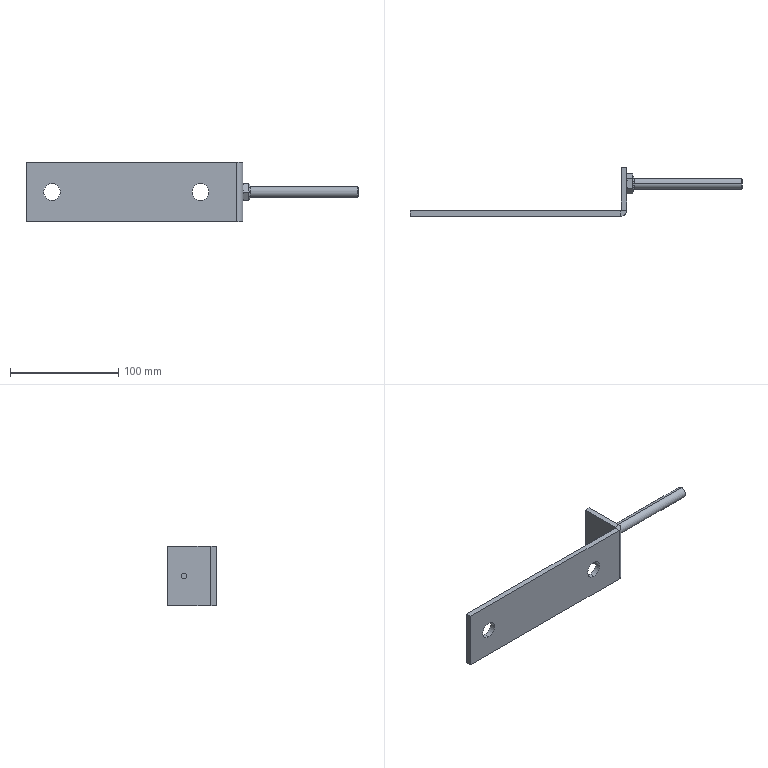Part | STEP file | Produce dryer driven tensioner plate | 2 solids | 44 faces | box 306.4 x 45 x 55 mm | volume 72873 mm3 | plane 22 | cylinder 10 | cone 10 | torus 2 | commonest cylinder face diameters 15.5 x4 5 x2 10 x2 1.473 x1 11.473 x1
STEP:
#1=CARTESIAN_POINT('',(195.,30.,-2.5));
#2=VERTEX_POINT('',#1);
#3=CARTESIAN_POINT('',(195.,30.,2.5));
#4=VERTEX_POINT('',#3);
#5=CARTESIAN_POINT('',(195.,30.,0.));
#6=DIRECTION('',(-1.,0.,0.));
#7=DIRECTION('',(0.,0.,1.));
#8=AXIS2_PLACEMENT_3D('',#5,#6,#7);
#9=CIRCLE('',#8,2.5);
#10=EDGE_CURVE('',#2,#4,#9,.T.);
#11=ORIENTED_EDGE('',*,*,#10,.T.);
#12=CARTESIAN_POINT('',(200.,30.,2.5));
#13=VERTEX_POINT('',#12);
#14=CARTESIAN_POINT('',(200.,30.,2.5));
#15=DIRECTION('',(1.,0.,0.));
#16=VECTOR('',#15,1000.);
#17=LINE('',#14,#16);
#18=EDGE_CURVE('',#4,#13,#17,.T.);
#19=ORIENTED_EDGE('',*,*,#18,.T.);
#20=CARTESIAN_POINT('',(200.,30.,-2.5));
#21=VERTEX_POINT('',#20);
#22=CARTESIAN_POINT('',(200.,30.,0.));
#23=DIRECTION('',(1.,0.,0.));
#24=DIRECTION('',(0.,0.,-1.));
#25=AXIS2_PLACEMENT_3D('',#22,#23,#24);
#26=CIRCLE('',#25,2.5);
#27=EDGE_CURVE('',#13,#21,#26,.T.);
#28=ORIENTED_EDGE('',*,*,#27,.T.);
#29=CARTESIAN_POINT('',(200.,30.,-2.5));
#30=DIRECTION('',(1.,0.,0.));
#31=VECTOR('',#30,1000.);
#32=LINE('',#29,#31);
#33=EDGE_CURVE('',#2,#21,#32,.T.);
#34=ORIENTED_EDGE('',*,*,#33,.F.);
#35=EDGE_LOOP('',(#11,#19,#28,#34));
#36=FACE_OUTER_BOUND('',#35,.T.);
#37=CARTESIAN_POINT('',(200.,30.,0.));
#38=DIRECTION('',(1.,0.,0.));
#39=DIRECTION('',(0.,0.,-1.));
#40=AXIS2_PLACEMENT_3D('',#37,#38,#39);
#41=CYLINDRICAL_SURFACE('',#40,2.5);
#42=ADVANCED_FACE('',(#36),#41,.F.);
#43=CARTESIAN_POINT('',(24.,0.,-7.75));
#44=VERTEX_POINT('',#43);
#45=CARTESIAN_POINT('',(24.,0.,7.75));
#46=VERTEX_POINT('',#45);
#47=CARTESIAN_POINT('',(24.,0.,0.));
#48=DIRECTION('',(0.,1.,0.));
#49=DIRECTION('',(0.,0.,1.));
#50=AXIS2_PLACEMENT_3D('',#47,#48,#49);
#51=CIRCLE('',#50,7.75);
#52=EDGE_CURVE('',#44,#46,#51,.T.);
#53=ORIENTED_EDGE('',*,*,#52,.F.);
#54=CARTESIAN_POINT('',(24.,5.,-7.75));
#55=VERTEX_POINT('',#54);
#56=CARTESIAN_POINT('',(24.,5.,-7.75));
#57=DIRECTION('',(0.,1.,0.));
#58=VECTOR('',#57,1000.);
#59=LINE('',#56,#58);
#60=EDGE_CURVE('',#44,#55,#59,.T.);
#61=ORIENTED_EDGE('',*,*,#60,.T.);
#62=CARTESIAN_POINT('',(24.,5.,7.75));
#63=VERTEX_POINT('',#62);
#64=CARTESIAN_POINT('',(24.,5.,0.));
#65=DIRECTION('',(0.,1.,0.));
#66=DIRECTION('',(0.,0.,1.));
#67=AXIS2_PLACEMENT_3D('',#64,#65,#66);
#68=CIRCLE('',#67,7.75);
#69=EDGE_CURVE('',#55,#63,#68,.T.);
#70=ORIENTED_EDGE('',*,*,#69,.T.);
#71=CARTESIAN_POINT('',(24.,5.,7.75));
#72=DIRECTION('',(0.,1.,0.));
#73=VECTOR('',#72,1000.);
#74=LINE('',#71,#73);
#75=EDGE_CURVE('',#46,#63,#74,.T.);
#76=ORIENTED_EDGE('',*,*,#75,.F.);
#77=EDGE_LOOP('',(#53,#61,#70,#76));
#78=FACE_OUTER_BOUND('',#77,.T.);
#79=CARTESIAN_POINT('',(24.,5.,0.));
#80=DIRECTION('',(0.,1.,0.));
#81=DIRECTION('',(0.,0.,1.));
#82=AXIS2_PLACEMENT_3D('',#79,#80,#81);
#83=CYLINDRICAL_SURFACE('',#82,7.75);
#84=ADVANCED_FACE('',(#78),#83,.F.);
#85=CARTESIAN_POINT('',(161.,0.,-7.75));
#86=VERTEX_POINT('',#85);
#87=CARTESIAN_POINT('',(161.,0.,7.75));
#88=VERTEX_POINT('',#87);
#89=CARTESIAN_POINT('',(161.,0.,0.));
#90=DIRECTION('',(0.,1.,0.));
#91=DIRECTION('',(0.,0.,1.));
#92=AXIS2_PLACEMENT_3D('',#89,#90,#91);
#93=CIRCLE('',#92,7.75);
#94=EDGE_CURVE('',#86,#88,#93,.T.);
#95=ORIENTED_EDGE('',*,*,#94,.F.);
#96=CARTESIAN_POINT('',(161.,5.,-7.75));
#97=VERTEX_POINT('',#96);
#98=CARTESIAN_POINT('',(161.,5.,-7.75));
#99=DIRECTION('',(0.,1.,0.));
#100=VECTOR('',#99,1000.);
#101=LINE('',#98,#100);
#102=EDGE_CURVE('',#86,#97,#101,.T.);
#103=ORIENTED_EDGE('',*,*,#102,.T.);
#104=CARTESIAN_POINT('',(161.,5.,7.75));
#105=VERTEX_POINT('',#104);
#106=CARTESIAN_POINT('',(161.,5.,0.));
#107=DIRECTION('',(0.,1.,0.));
#108=DIRECTION('',(0.,0.,1.));
#109=AXIS2_PLACEMENT_3D('',#106,#107,#108);
#110=CIRCLE('',#109,7.75);
#111=EDGE_CURVE('',#97,#105,#110,.T.);
#112=ORIENTED_EDGE('',*,*,#111,.T.);
#113=CARTESIAN_POINT('',(161.,5.,7.75));
#114=DIRECTION('',(0.,1.,0.));
#115=VECTOR('',#114,1000.);
#116=LINE('',#113,#115);
#117=EDGE_CURVE('',#88,#105,#116,.T.);
#118=ORIENTED_EDGE('',*,*,#117,.F.);
#119=EDGE_LOOP('',(#95,#103,#112,#118));
#120=FACE_OUTER_BOUND('',#119,.T.);
#121=CARTESIAN_POINT('',(161.,5.,0.));
#122=DIRECTION('',(0.,1.,0.));
#123=DIRECTION('',(0.,0.,1.));
#124=AXIS2_PLACEMENT_3D('',#121,#122,#123);
#125=CYLINDRICAL_SURFACE('',#124,7.75);
#126=ADVANCED_FACE('',(#120),#125,.F.);
#127=CARTESIAN_POINT('',(194.263,0.,27.5));
#128=VERTEX_POINT('',#127);
#129=CARTESIAN_POINT('',(194.263,5.,27.5));
#130=VERTEX_POINT('',#129);
#131=CARTESIAN_POINT('',(194.263,0.,27.5));
#132=DIRECTION('',(0.,1.,0.));
#133=VECTOR('',#132,1000.);
#134=LINE('',#131,#133);
#135=EDGE_CURVE('',#128,#130,#134,.T.);
#136=ORIENTED_EDGE('',*,*,#135,.F.);
#137=CARTESIAN_POINT('',(200.,5.737,27.5));
#138=VERTEX_POINT('',#137);
#139=CARTESIAN_POINT('',(194.263,5.737,27.5));
#140=DIRECTION('',(0.,0.,1.));
#141=DIRECTION('',(-1.,0.,0.));
#142=AXIS2_PLACEMENT_3D('',#139,#140,#141);
#143=CIRCLE('',#142,5.737);
#144=EDGE_CURVE('',#128,#138,#143,.T.);
#145=ORIENTED_EDGE('',*,*,#144,.T.);
#146=CARTESIAN_POINT('',(195.,5.737,27.5));
#147=VERTEX_POINT('',#146);
#148=CARTESIAN_POINT('',(195.,5.737,27.5));
#149=DIRECTION('',(1.,0.,0.));
#150=VECTOR('',#149,1000.);
#151=LINE('',#148,#150);
#152=EDGE_CURVE('',#147,#138,#151,.T.);
#153=ORIENTED_EDGE('',*,*,#152,.F.);
#154=CARTESIAN_POINT('',(194.263,5.737,27.5));
#155=DIRECTION('',(0.,0.,1.));
#156=DIRECTION('',(1.,0.,0.));
#157=AXIS2_PLACEMENT_3D('',#154,#155,#156);
#158=CIRCLE('',#157,0.7366);
#159=EDGE_CURVE('',#130,#147,#158,.T.);
#160=ORIENTED_EDGE('',*,*,#159,.F.);
#161=EDGE_LOOP('',(#136,#145,#153,#160));
#162=FACE_OUTER_BOUND('',#161,.T.);
#163=CARTESIAN_POINT('',(194.263,0.,27.5));
#164=DIRECTION('',(0.,0.,1.));
#165=DIRECTION('',(1.,0.,0.));
#166=AXIS2_PLACEMENT_3D('',#163,#164,#165);
#167=PLANE('',#166);
#168=ADVANCED_FACE('',(#162),#167,.T.);
#169=CARTESIAN_POINT('',(0.,0.,27.5));
#170=VERTEX_POINT('',#169);
#171=CARTESIAN_POINT('',(0.,0.,27.5));
#172=DIRECTION('',(1.,0.,0.));
#173=VECTOR('',#172,1000.);
#174=LINE('',#171,#173);
#175=EDGE_CURVE('',#170,#128,#174,.T.);
#176=ORIENTED_EDGE('',*,*,#175,.T.);
#177=ORIENTED_EDGE('',*,*,#135,.T.);
#178=CARTESIAN_POINT('',(0.,5.,27.5));
#179=VERTEX_POINT('',#178);
#180=CARTESIAN_POINT('',(0.,5.,27.5));
#181=DIRECTION('',(1.,0.,0.));
#182=VECTOR('',#181,1000.);
#183=LINE('',#180,#182);
#184=EDGE_CURVE('',#179,#130,#183,.T.);
#185=ORIENTED_EDGE('',*,*,#184,.F.);
#186=CARTESIAN_POINT('',(0.,0.,27.5));
#187=DIRECTION('',(0.,1.,0.));
#188=VECTOR('',#187,1000.);
#189=LINE('',#186,#188);
#190=EDGE_CURVE('',#170,#179,#189,.T.);
#191=ORIENTED_EDGE('',*,*,#190,.F.);
#192=EDGE_LOOP('',(#176,#177,#185,#191));
#193=FACE_OUTER_BOUND('',#192,.T.);
#194=CARTESIAN_POINT('',(195.,5.737,27.5));
#195=DIRECTION('',(0.,0.,1.));
#196=DIRECTION('',(1.,0.,0.));
#197=AXIS2_PLACEMENT_3D('',#194,#195,#196);
#198=PLANE('',#197);
#199=ADVANCED_FACE('',(#193),#198,.T.);
#200=CARTESIAN_POINT('',(200.,5.737,-27.5));
#201=VERTEX_POINT('',#200);
#202=CARTESIAN_POINT('',(195.,5.737,-27.5));
#203=VERTEX_POINT('',#202);
#204=CARTESIAN_POINT('',(200.,5.737,-27.5));
#205=DIRECTION('',(-1.,0.,0.));
#206=VECTOR('',#205,1000.);
#207=LINE('',#204,#206);
#208=EDGE_CURVE('',#201,#203,#207,.T.);
#209=ORIENTED_EDGE('',*,*,#208,.F.);
#210=CARTESIAN_POINT('',(194.263,0.,-27.5));
#211=VERTEX_POINT('',#210);
#212=CARTESIAN_POINT('',(194.263,5.737,-27.5));
#213=DIRECTION('',(0.,0.,1.));
#214=DIRECTION('',(-1.,0.,0.));
#215=AXIS2_PLACEMENT_3D('',#212,#213,#214);
#216=CIRCLE('',#215,5.737);
#217=EDGE_CURVE('',#211,#201,#216,.T.);
#218=ORIENTED_EDGE('',*,*,#217,.F.);
#219=CARTESIAN_POINT('',(194.263,5.,-27.5));
#220=VERTEX_POINT('',#219);
#221=CARTESIAN_POINT('',(194.263,5.,-27.5));
#222=DIRECTION('',(0.,-1.,0.));
#223=VECTOR('',#222,1000.);
#224=LINE('',#221,#223);
#225=EDGE_CURVE('',#220,#211,#224,.T.);
#226=ORIENTED_EDGE('',*,*,#225,.F.);
#227=CARTESIAN_POINT('',(194.263,5.737,-27.5));
#228=DIRECTION('',(0.,0.,1.));
#229=DIRECTION('',(1.,0.,0.));
#230=AXIS2_PLACEMENT_3D('',#227,#228,#229);
#231=CIRCLE('',#230,0.7366);
#232=EDGE_CURVE('',#220,#203,#231,.T.);
#233=ORIENTED_EDGE('',*,*,#232,.T.);
#234=EDGE_LOOP('',(#209,#218,#226,#233));
#235=FACE_OUTER_BOUND('',#234,.T.);
#236=CARTESIAN_POINT('',(200.,5.737,-27.5));
#237=DIRECTION('',(0.,0.,-1.));
#238=DIRECTION('',(-1.,0.,0.));
#239=AXIS2_PLACEMENT_3D('',#236,#237,#238);
#240=PLANE('',#239);
#241=ADVANCED_FACE('',(#235),#240,.T.);
#242=CARTESIAN_POINT('',(200.,45.,-27.5));
#243=VERTEX_POINT('',#242);
#244=CARTESIAN_POINT('',(200.,0.,-27.5));
#245=DIRECTION('',(0.,1.,0.));
#246=VECTOR('',#245,1000.);
#247=LINE('',#244,#246);
#248=EDGE_CURVE('',#201,#243,#247,.T.);
#249=ORIENTED_EDGE('',*,*,#248,.F.);
#250=ORIENTED_EDGE('',*,*,#208,.T.);
#251=CARTESIAN_POINT('',(195.,45.,-27.5));
#252=VERTEX_POINT('',#251);
#253=CARTESIAN_POINT('',(195.,0.,-27.5));
#254=DIRECTION('',(0.,1.,0.));
#255=VECTOR('',#254,1000.);
#256=LINE('',#253,#255);
#257=EDGE_CURVE('',#203,#252,#256,.T.);
#258=ORIENTED_EDGE('',*,*,#257,.T.);
#259=CARTESIAN_POINT('',(195.,45.,-27.5));
#260=DIRECTION('',(1.,0.,0.));
#261=VECTOR('',#260,1000.);
#262=LINE('',#259,#261);
#263=EDGE_CURVE('',#252,#243,#262,.T.);
#264=ORIENTED_EDGE('',*,*,#263,.T.);
#265=EDGE_LOOP('',(#249,#250,#258,#264));
#266=FACE_OUTER_BOUND('',#265,.T.);
#267=CARTESIAN_POINT('',(194.263,5.,-27.5));
#268=DIRECTION('',(0.,0.,-1.));
#269=DIRECTION('',(-1.,0.,0.));
#270=AXIS2_PLACEMENT_3D('',#267,#268,#269);
#271=PLANE('',#270);
#272=ADVANCED_FACE('',(#266),#271,.T.);
#273=CARTESIAN_POINT('',(200.,30.,0.));
#274=DIRECTION('',(1.,0.,0.));
#275=DIRECTION('',(0.,0.,-1.));
#276=AXIS2_PLACEMENT_3D('',#273,#274,#275);
#277=CIRCLE('',#276,2.5);
#278=EDGE_CURVE('',#21,#13,#277,.T.);
#279=ORIENTED_EDGE('',*,*,#278,.F.);
#280=ORIENTED_EDGE('',*,*,#27,.F.);
#281=EDGE_LOOP('',(#279,#280));
#282=FACE_BOUND('',#281,.T.);
#283=ORIENTED_EDGE('',*,*,#248,.T.);
#284=CARTESIAN_POINT('',(200.,45.,27.5));
#285=VERTEX_POINT('',#284);
#286=CARTESIAN_POINT('',(200.,45.,27.5));
#287=DIRECTION('',(0.,0.,-1.));
#288=VECTOR('',#287,1000.);
#289=LINE('',#286,#288);
#290=EDGE_CURVE('',#285,#243,#289,.T.);
#291=ORIENTED_EDGE('',*,*,#290,.F.);
#292=CARTESIAN_POINT('',(200.,0.,27.5));
#293=DIRECTION('',(0.,1.,0.));
#294=VECTOR('',#293,1000.);
#295=LINE('',#292,#294);
#296=EDGE_CURVE('',#138,#285,#295,.T.);
#297=ORIENTED_EDGE('',*,*,#296,.F.);
#298=CARTESIAN_POINT('',(200.,5.737,27.5));
#299=DIRECTION('',(0.,0.,-1.));
#300=VECTOR('',#299,1000.);
#301=LINE('',#298,#300);
#302=EDGE_CURVE('',#138,#201,#301,.T.);
#303=ORIENTED_EDGE('',*,*,#302,.T.);
#304=EDGE_LOOP('',(#283,#291,#297,#303));
#305=FACE_OUTER_BOUND('',#304,.T.);
#306=CARTESIAN_POINT('',(200.,0.,27.5));
#307=DIRECTION('',(-1.,0.,0.));
#308=DIRECTION('',(0.,0.,1.));
#309=AXIS2_PLACEMENT_3D('',#306,#307,#308);
#310=PLANE('',#309);
#311=ADVANCED_FACE('',(#282,#305),#310,.F.);
#312=ORIENTED_EDGE('',*,*,#263,.F.);
#313=CARTESIAN_POINT('',(195.,45.,27.5));
#314=VERTEX_POINT('',#313);
#315=CARTESIAN_POINT('',(195.,45.,27.5));
#316=DIRECTION('',(0.,0.,-1.));
#317=VECTOR('',#316,1000.);
#318=LINE('',#315,#317);
#319=EDGE_CURVE('',#314,#252,#318,.T.);
#320=ORIENTED_EDGE('',*,*,#319,.F.);
#321=CARTESIAN_POINT('',(195.,45.,27.5));
#322=DIRECTION('',(1.,0.,0.));
#323=VECTOR('',#322,1000.);
#324=LINE('',#321,#323);
#325=EDGE_CURVE('',#314,#285,#324,.T.);
#326=ORIENTED_EDGE('',*,*,#325,.T.);
#327=ORIENTED_EDGE('',*,*,#290,.T.);
#328=EDGE_LOOP('',(#312,#320,#326,#327));
#329=FACE_OUTER_BOUND('',#328,.T.);
#330=CARTESIAN_POINT('',(195.,45.,27.5));
#331=DIRECTION('',(0.,1.,0.));
#332=DIRECTION('',(0.,0.,1.));
#333=AXIS2_PLACEMENT_3D('',#330,#331,#332);
#334=PLANE('',#333);
#335=ADVANCED_FACE('',(#329),#334,.T.);
#336=ORIENTED_EDGE('',*,*,#10,.F.);
#337=CARTESIAN_POINT('',(195.,30.,0.));
#338=DIRECTION('',(-1.,0.,0.));
#339=DIRECTION('',(0.,0.,1.));
#340=AXIS2_PLACEMENT_3D('',#337,#338,#339);
#341=CIRCLE('',#340,2.5);
#342=EDGE_CURVE('',#4,#2,#341,.T.);
#343=ORIENTED_EDGE('',*,*,#342,.F.);
#344=EDGE_LOOP('',(#336,#343));
#345=FACE_BOUND('',#344,.T.);
#346=ORIENTED_EDGE('',*,*,#257,.F.);
#347=CARTESIAN_POINT('',(195.,5.737,27.5));
#348=DIRECTION('',(0.,0.,-1.));
#349=VECTOR('',#348,1000.);
#350=LINE('',#347,#349);
#351=EDGE_CURVE('',#147,#203,#350,.T.);
#352=ORIENTED_EDGE('',*,*,#351,.F.);
#353=CARTESIAN_POINT('',(195.,0.,27.5));
#354=DIRECTION('',(0.,1.,0.));
#355=VECTOR('',#354,1000.);
#356=LINE('',#353,#355);
#357=EDGE_CURVE('',#147,#314,#356,.T.);
#358=ORIENTED_EDGE('',*,*,#357,.T.);
#359=ORIENTED_EDGE('',*,*,#319,.T.);
#360=EDGE_LOOP('',(#346,#352,#358,#359));
#361=FACE_OUTER_BOUND('',#360,.T.);
#362=CARTESIAN_POINT('',(195.,0.,27.5));
#363=DIRECTION('',(-1.,0.,0.));
#364=DIRECTION('',(0.,0.,1.));
#365=AXIS2_PLACEMENT_3D('',#362,#363,#364);
#366=PLANE('',#365);
#367=ADVANCED_FACE('',(#345,#361),#366,.T.);
#368=ORIENTED_EDGE('',*,*,#232,.F.);
#369=CARTESIAN_POINT('',(194.263,5.,27.5));
#370=DIRECTION('',(0.,0.,-1.));
#371=VECTOR('',#370,1000.);
#372=LINE('',#369,#371);
#373=EDGE_CURVE('',#130,#220,#372,.T.);
#374=ORIENTED_EDGE('',*,*,#373,.F.);
#375=ORIENTED_EDGE('',*,*,#159,.T.);
#376=ORIENTED_EDGE('',*,*,#351,.T.);
#377=EDGE_LOOP('',(#368,#374,#375,#376));
#378=FACE_OUTER_BOUND('',#377,.T.);
#379=CARTESIAN_POINT('',(194.263,5.737,27.5));
#380=DIRECTION('',(0.,0.,-1.));
#381=DIRECTION('',(-1.,0.,0.));
#382=AXIS2_PLACEMENT_3D('',#379,#380,#381);
#383=CYLINDRICAL_SURFACE('',#382,0.7366);
#384=ADVANCED_FACE('',(#378),#383,.F.);
#385=CARTESIAN_POINT('',(24.,5.,0.));
#386=DIRECTION('',(0.,1.,0.));
#387=DIRECTION('',(0.,0.,1.));
#388=AXIS2_PLACEMENT_3D('',#385,#386,#387);
#389=CIRCLE('',#388,7.75);
#390=EDGE_CURVE('',#63,#55,#389,.T.);
#391=ORIENTED_EDGE('',*,*,#390,.F.);
#392=ORIENTED_EDGE('',*,*,#69,.F.);
#393=EDGE_LOOP('',(#391,#392));
#394=FACE_BOUND('',#393,.T.);
#395=CARTESIAN_POINT('',(161.,5.,0.));
#396=DIRECTION('',(0.,1.,0.));
#397=DIRECTION('',(0.,0.,1.));
#398=AXIS2_PLACEMENT_3D('',#395,#396,#397);
#399=CIRCLE('',#398,7.75);
#400=EDGE_CURVE('',#105,#97,#399,.T.);
#401=ORIENTED_EDGE('',*,*,#400,.F.);
#402=ORIENTED_EDGE('',*,*,#111,.F.);
#403=EDGE_LOOP('',(#401,#402));
#404=FACE_BOUND('',#403,.T.);
#405=CARTESIAN_POINT('',(0.,5.,-27.5));
#406=VERTEX_POINT('',#405);
#407=CARTESIAN_POINT('',(0.,5.,-27.5));
#408=DIRECTION('',(1.,0.,0.));
#409=VECTOR('',#408,1000.);
#410=LINE('',#407,#409);
#411=EDGE_CURVE('',#406,#220,#410,.T.);
#412=ORIENTED_EDGE('',*,*,#411,.F.);
#413=CARTESIAN_POINT('',(0.,5.,27.5));
#414=DIRECTION('',(0.,0.,-1.));
#415=VECTOR('',#414,1000.);
#416=LINE('',#413,#415);
#417=EDGE_CURVE('',#179,#406,#416,.T.);
#418=ORIENTED_EDGE('',*,*,#417,.F.);
#419=ORIENTED_EDGE('',*,*,#184,.T.);
#420=ORIENTED_EDGE('',*,*,#373,.T.);
#421=EDGE_LOOP('',(#412,#418,#419,#420));
#422=FACE_OUTER_BOUND('',#421,.T.);
#423=CARTESIAN_POINT('',(0.,5.,27.5));
#424=DIRECTION('',(0.,1.,0.));
#425=DIRECTION('',(0.,0.,1.));
#426=AXIS2_PLACEMENT_3D('',#423,#424,#425);
#427=PLANE('',#426);
#428=ADVANCED_FACE('',(#394,#404,#422),#427,.T.);
#429=CARTESIAN_POINT('',(0.,0.,-27.5));
#430=VERTEX_POINT('',#429);
#431=CARTESIAN_POINT('',(0.,0.,-27.5));
#432=DIRECTION('',(0.,1.,0.));
#433=VECTOR('',#432,1000.);
#434=LINE('',#431,#433);
#435=EDGE_CURVE('',#430,#406,#434,.T.);
#436=ORIENTED_EDGE('',*,*,#435,.F.);
#437=CARTESIAN_POINT('',(0.,0.,27.5));
#438=DIRECTION('',(0.,0.,-1.));
#439=VECTOR('',#438,1000.);
#440=LINE('',#437,#439);
#441=EDGE_CURVE('',#170,#430,#440,.T.);
#442=ORIENTED_EDGE('',*,*,#441,.F.);
#443=ORIENTED_EDGE('',*,*,#190,.T.);
#444=ORIENTED_EDGE('',*,*,#417,.T.);
#445=EDGE_LOOP('',(#436,#442,#443,#444));
#446=FACE_OUTER_BOUND('',#445,.T.);
#447=CARTESIAN_POINT('',(0.,0.,27.5));
#448=DIRECTION('',(-1.,0.,0.));
#449=DIRECTION('',(0.,0.,1.));
#450=AXIS2_PLACEMENT_3D('',#447,#448,#449);
#451=PLANE('',#450);
#452=ADVANCED_FACE('',(#446),#451,.T.);
#453=CARTESIAN_POINT('',(24.,0.,0.));
#454=DIRECTION('',(0.,1.,0.));
#455=DIRECTION('',(0.,0.,1.));
#456=AXIS2_PLACEMENT_3D('',#453,#454,#455);
#457=CIRCLE('',#456,7.75);
#458=EDGE_CURVE('',#46,#44,#457,.T.);
#459=ORIENTED_EDGE('',*,*,#458,.T.);
#460=ORIENTED_EDGE('',*,*,#52,.T.);
#461=EDGE_LOOP('',(#459,#460));
#462=FACE_BOUND('',#461,.T.);
#463=CARTESIAN_POINT('',(161.,0.,0.));
#464=DIRECTION('',(0.,1.,0.));
#465=DIRECTION('',(0.,0.,1.));
#466=AXIS2_PLACEMENT_3D('',#463,#464,#465);
#467=CIRCLE('',#466,7.75);
#468=EDGE_CURVE('',#88,#86,#467,.T.);
#469=ORIENTED_EDGE('',*,*,#468,.T.);
#470=ORIENTED_EDGE('',*,*,#94,.T.);
#471=EDGE_LOOP('',(#469,#470));
#472=FACE_BOUND('',#471,.T.);
#473=CARTESIAN_POINT('',(0.,0.,-27.5));
#474=DIRECTION('',(1.,0.,0.));
#475=VECTOR('',#474,1000.);
#476=LINE('',#473,#475);
#477=EDGE_CURVE('',#430,#211,#476,.T.);
#478=ORIENTED_EDGE('',*,*,#477,.T.);
#479=CARTESIAN_POINT('',(194.263,0.,27.5));
#480=DIRECTION('',(0.,0.,-1.));
#481=VECTOR('',#480,1000.);
#482=LINE('',#479,#481);
#483=EDGE_CURVE('',#128,#211,#482,.T.);
#484=ORIENTED_EDGE('',*,*,#483,.F.);
#485=ORIENTED_EDGE('',*,*,#175,.F.);
#486=ORIENTED_EDGE('',*,*,#441,.T.);
#487=EDGE_LOOP('',(#478,#484,#485,#486));
#488=FACE_OUTER_BOUND('',#487,.T.);
#489=CARTESIAN_POINT('',(0.,0.,27.5));
#490=DIRECTION('',(0.,1.,0.));
#491=DIRECTION('',(0.,0.,1.));
#492=AXIS2_PLACEMENT_3D('',#489,#490,#491);
#493=PLANE('',#492);
#494=ADVANCED_FACE('',(#462,#472,#488),#493,.F.);
#495=ORIENTED_EDGE('',*,*,#217,.T.);
#496=ORIENTED_EDGE('',*,*,#302,.F.);
#497=ORIENTED_EDGE('',*,*,#144,.F.);
#498=ORIENTED_EDGE('',*,*,#483,.T.);
#499=EDGE_LOOP('',(#495,#496,#497,#498));
#500=FACE_OUTER_BOUND('',#499,.T.);
#501=CARTESIAN_POINT('',(194.263,5.737,27.5));
#502=DIRECTION('',(0.,0.,-1.));
#503=DIRECTION('',(-1.,0.,0.));
#504=AXIS2_PLACEMENT_3D('',#501,#502,#503);
#505=CYLINDRICAL_SURFACE('',#504,5.737);
#506=ADVANCED_FACE('',(#500),#505,.T.);
#507=ORIENTED_EDGE('',*,*,#296,.T.);
#508=ORIENTED_EDGE('',*,*,#325,.F.);
#509=ORIENTED_EDGE('',*,*,#357,.F.);
#510=ORIENTED_EDGE('',*,*,#152,.T.);
#511=EDGE_LOOP('',(#507,#508,#509,#510));
#512=FACE_OUTER_BOUND('',#511,.T.);
#513=CARTESIAN_POINT('',(194.263,5.737,27.5));
#514=DIRECTION('',(0.,0.,1.));
#515=DIRECTION('',(1.,0.,0.));
#516=AXIS2_PLACEMENT_3D('',#513,#514,#515);
#517=PLANE('',#516);
#518=ADVANCED_FACE('',(#512),#517,.T.);
#519=ORIENTED_EDGE('',*,*,#411,.T.);
#520=ORIENTED_EDGE('',*,*,#225,.T.);
#521=ORIENTED_EDGE('',*,*,#477,.F.);
#522=ORIENTED_EDGE('',*,*,#435,.T.);
#523=EDGE_LOOP('',(#519,#520,#521,#522));
#524=FACE_OUTER_BOUND('',#523,.T.);
#525=CARTESIAN_POINT('',(194.263,5.737,-27.5));
#526=DIRECTION('',(0.,0.,1.));
#527=DIRECTION('',(1.,0.,0.));
#528=AXIS2_PLACEMENT_3D('',#525,#526,#527);
#529=PLANE('',#528);
#530=ADVANCED_FACE('',(#524),#529,.F.);
#531=ORIENTED_EDGE('',*,*,#102,.F.);
#532=ORIENTED_EDGE('',*,*,#468,.F.);
#533=ORIENTED_EDGE('',*,*,#117,.T.);
#534=ORIENTED_EDGE('',*,*,#400,.T.);
#535=EDGE_LOOP('',(#531,#532,#533,#534));
#536=FACE_OUTER_BOUND('',#535,.T.);
#537=CARTESIAN_POINT('',(161.,5.,0.));
#538=DIRECTION('',(0.,1.,0.));
#539=DIRECTION('',(0.,0.,1.));
#540=AXIS2_PLACEMENT_3D('',#537,#538,#539);
#541=CYLINDRICAL_SURFACE('',#540,7.75);
#542=ADVANCED_FACE('',(#536),#541,.F.);
#543=ORIENTED_EDGE('',*,*,#60,.F.);
#544=ORIENTED_EDGE('',*,*,#458,.F.);
#545=ORIENTED_EDGE('',*,*,#75,.T.);
#546=ORIENTED_EDGE('',*,*,#390,.T.);
#547=EDGE_LOOP('',(#543,#544,#545,#546));
#548=FACE_OUTER_BOUND('',#547,.T.);
#549=CARTESIAN_POINT('',(24.,5.,0.));
#550=DIRECTION('',(0.,1.,0.));
#551=DIRECTION('',(0.,0.,1.));
#552=AXIS2_PLACEMENT_3D('',#549,#550,#551);
#553=CYLINDRICAL_SURFACE('',#552,7.75);
#554=ADVANCED_FACE('',(#548),#553,.F.);
#555=ORIENTED_EDGE('',*,*,#18,.F.);
#556=ORIENTED_EDGE('',*,*,#342,.T.);
#557=ORIENTED_EDGE('',*,*,#33,.T.);
#558=ORIENTED_EDGE('',*,*,#278,.T.);
#559=EDGE_LOOP('',(#555,#556,#557,#558));
#560=FACE_OUTER_BOUND('',#559,.T.);
#561=CARTESIAN_POINT('',(200.,30.,0.));
#562=DIRECTION('',(1.,0.,0.));
#563=DIRECTION('',(0.,0.,-1.));
#564=AXIS2_PLACEMENT_3D('',#561,#562,#563);
#565=CYLINDRICAL_SURFACE('',#564,2.5);
#566=ADVANCED_FACE('',(#560),#565,.F.);
#567=CLOSED_SHELL('',(#42,#84,#126,#168,#199,#241,#272,#311,#335,#367,#384,#428,#452,#494,#506,#518,#530,#542,#554,#566));
#568=MANIFOLD_SOLID_BREP('',#567);
#569=CARTESIAN_POINT('',(206.4,30.,7.215));
#570=VERTEX_POINT('',#569);
#571=CARTESIAN_POINT('',(206.4,30.,-7.215));
#572=VERTEX_POINT('',#571);
#573=CARTESIAN_POINT('',(206.4,30.,0.));
#574=DIRECTION('',(-1.,0.,0.));
#575=DIRECTION('',(0.,0.,1.));
#576=AXIS2_PLACEMENT_3D('',#573,#574,#575);
#577=CIRCLE('',#576,7.215);
#578=EDGE_CURVE('',#570,#572,#577,.T.);
#579=ORIENTED_EDGE('',*,*,#578,.T.);
#580=CARTESIAN_POINT('',(205.8,30.,-7.815));
#581=VERTEX_POINT('',#580);
#582=CARTESIAN_POINT('',(205.8,30.,-7.815));
#583=DIRECTION('',(-0.7071,0.,-0.7071));
#584=VECTOR('',#583,1000.);
#585=LINE('',#582,#584);
#586=EDGE_CURVE('',#572,#581,#585,.T.);
#587=ORIENTED_EDGE('',*,*,#586,.T.);
#588=CARTESIAN_POINT('',(205.8,30.,7.815));
#589=VERTEX_POINT('',#588);
#590=CARTESIAN_POINT('',(205.8,30.,0.));
#591=DIRECTION('',(-1.,0.,0.));
#592=DIRECTION('',(0.,0.,1.));
#593=AXIS2_PLACEMENT_3D('',#590,#591,#592);
#594=CIRCLE('',#593,7.815);
#595=EDGE_CURVE('',#589,#581,#594,.T.);
#596=ORIENTED_EDGE('',*,*,#595,.F.);
#597=CARTESIAN_POINT('',(205.8,30.,7.815));
#598=DIRECTION('',(-0.7071,0.,0.7071));
#599=VECTOR('',#598,1000.);
#600=LINE('',#597,#599);
#601=EDGE_CURVE('',#570,#589,#600,.T.);
#602=ORIENTED_EDGE('',*,*,#601,.F.);
#603=EDGE_LOOP('',(#579,#587,#596,#602));
#604=FACE_OUTER_BOUND('',#603,.T.);
#605=CARTESIAN_POINT('',(205.8,30.,0.));
#606=DIRECTION('',(-1.,0.,0.));
#607=DIRECTION('',(0.,0.,1.));
#608=AXIS2_PLACEMENT_3D('',#605,#606,#607);
#609=CONICAL_SURFACE('',#608,7.815,0.7854);
#610=ADVANCED_FACE('',(#604),#609,.T.);
#611=CARTESIAN_POINT('',(306.4,30.,-4.444));
#612=VERTEX_POINT('',#611);
#613=CARTESIAN_POINT('',(306.4,30.,4.444));
#614=VERTEX_POINT('',#613);
#615=CARTESIAN_POINT('',(306.4,30.,0.));
#616=DIRECTION('',(1.,0.,0.));
#617=DIRECTION('',(0.,0.,1.));
#618=AXIS2_PLACEMENT_3D('',#615,#616,#617);
#619=CIRCLE('',#618,4.444);
#620=EDGE_CURVE('',#612,#614,#619,.T.);
#621=ORIENTED_EDGE('',*,*,#620,.F.);
#622=CARTESIAN_POINT('',(305.844,30.,-5.));
#623=VERTEX_POINT('',#622);
#624=CARTESIAN_POINT('',(305.844,30.,-5.));
#625=DIRECTION('',(-0.7071,0.,-0.7071));
#626=VECTOR('',#625,1000.);
#627=LINE('',#624,#626);
#628=EDGE_CURVE('',#612,#623,#627,.T.);
#629=ORIENTED_EDGE('',*,*,#628,.T.);
#630=CARTESIAN_POINT('',(305.844,30.,5.));
#631=VERTEX_POINT('',#630);
#632=CARTESIAN_POINT('',(305.844,30.,0.));
#633=DIRECTION('',(-1.,0.,0.));
#634=DIRECTION('',(0.,0.,1.));
#635=AXIS2_PLACEMENT_3D('',#632,#633,#634);
#636=CIRCLE('',#635,5.);
#637=EDGE_CURVE('',#631,#623,#636,.T.);
#638=ORIENTED_EDGE('',*,*,#637,.F.);
#639=CARTESIAN_POINT('',(305.844,30.,5.));
#640=DIRECTION('',(-0.7071,0.,0.7071));
#641=VECTOR('',#640,1000.);
#642=LINE('',#639,#641);
#643=EDGE_CURVE('',#614,#631,#642,.T.);
#644=ORIENTED_EDGE('',*,*,#643,.F.);
#645=EDGE_LOOP('',(#621,#629,#638,#644));
#646=FACE_OUTER_BOUND('',#645,.T.);
#647=CARTESIAN_POINT('',(305.844,30.,0.));
#648=DIRECTION('',(-1.,0.,0.));
#649=DIRECTION('',(0.,0.,1.));
#650=AXIS2_PLACEMENT_3D('',#647,#648,#649);
#651=CONICAL_SURFACE('',#650,5.,0.7854);
#652=ADVANCED_FACE('',(#646),#651,.T.);
#653=ORIENTED_EDGE('',*,*,#637,.T.);
#654=CARTESIAN_POINT('',(207.,30.,-5.));
#655=VERTEX_POINT('',#654);
#656=CARTESIAN_POINT('',(206.4,30.,-5.));
#657=DIRECTION('',(-1.,0.,0.));
#658=VECTOR('',#657,1000.);
#659=LINE('',#656,#658);
#660=EDGE_CURVE('',#623,#655,#659,.T.);
#661=ORIENTED_EDGE('',*,*,#660,.T.);
#662=CARTESIAN_POINT('',(207.,30.,5.));
#663=VERTEX_POINT('',#662);
#664=CARTESIAN_POINT('',(207.,30.,0.));
#665=DIRECTION('',(-1.,0.,0.));
#666=DIRECTION('',(0.,0.,1.));
#667=AXIS2_PLACEMENT_3D('',#664,#665,#666);
#668=CIRCLE('',#667,5.);
#669=EDGE_CURVE('',#663,#655,#668,.T.);
#670=ORIENTED_EDGE('',*,*,#669,.F.);
#671=CARTESIAN_POINT('',(206.4,30.,5.));
#672=DIRECTION('',(-1.,0.,0.));
#673=VECTOR('',#672,1000.);
#674=LINE('',#671,#673);
#675=EDGE_CURVE('',#631,#663,#674,.T.);
#676=ORIENTED_EDGE('',*,*,#675,.F.);
#677=EDGE_LOOP('',(#653,#661,#670,#676));
#678=FACE_OUTER_BOUND('',#677,.T.);
#679=CARTESIAN_POINT('',(206.4,30.,0.));
#680=DIRECTION('',(-1.,0.,0.));
#681=DIRECTION('',(0.,0.,1.));
#682=AXIS2_PLACEMENT_3D('',#679,#680,#681);
#683=CYLINDRICAL_SURFACE('',#682,5.);
#684=ADVANCED_FACE('',(#678),#683,.T.);
#685=CARTESIAN_POINT('',(206.4,30.,-5.6));
#686=VERTEX_POINT('',#685);
#687=CARTESIAN_POINT('',(206.4,30.,5.6));
#688=VERTEX_POINT('',#687);
#689=CARTESIAN_POINT('',(206.4,30.,0.));
#690=DIRECTION('',(-1.,0.,0.));
#691=DIRECTION('',(0.,0.,1.));
#692=AXIS2_PLACEMENT_3D('',#689,#690,#691);
#693=CIRCLE('',#692,5.6);
#694=EDGE_CURVE('',#686,#688,#693,.T.);
#695=ORIENTED_EDGE('',*,*,#694,.F.);
#696=CARTESIAN_POINT('',(207.,30.,-5.6));
#697=DIRECTION('',(0.,1.,0.));
#698=DIRECTION('',(0.,0.,1.));
#699=AXIS2_PLACEMENT_3D('',#696,#697,#698);
#700=CIRCLE('',#699,0.6);
#701=EDGE_CURVE('',#686,#655,#700,.T.);
#702=ORIENTED_EDGE('',*,*,#701,.T.);
#703=CARTESIAN_POINT('',(207.,30.,0.));
#704=DIRECTION('',(-1.,0.,0.));
#705=DIRECTION('',(0.,0.,1.));
#706=AXIS2_PLACEMENT_3D('',#703,#704,#705);
#707=CIRCLE('',#706,5.);
#708=EDGE_CURVE('',#655,#663,#707,.T.);
#709=ORIENTED_EDGE('',*,*,#708,.T.);
#710=CARTESIAN_POINT('',(207.,30.,5.6));
#711=DIRECTION('',(0.,-1.,0.));
#712=DIRECTION('',(0.,0.,-1.));
#713=AXIS2_PLACEMENT_3D('',#710,#711,#712);
#714=CIRCLE('',#713,0.6);
#715=EDGE_CURVE('',#688,#663,#714,.T.);
#716=ORIENTED_EDGE('',*,*,#715,.F.);
#717=EDGE_LOOP('',(#695,#702,#709,#716));
#718=FACE_OUTER_BOUND('',#717,.T.);
#719=CARTESIAN_POINT('',(207.,30.,0.));
#720=DIRECTION('',(-1.,0.,0.));
#721=DIRECTION('',(0.,0.,1.));
#722=AXIS2_PLACEMENT_3D('',#719,#720,#721);
#723=TOROIDAL_SURFACE('',#722,5.6,0.6);
#724=ADVANCED_FACE('',(#718),#723,.F.);
#725=CARTESIAN_POINT('',(206.4,30.,0.));
#726=DIRECTION('',(-1.,0.,0.));
#727=DIRECTION('',(0.,0.,1.));
#728=AXIS2_PLACEMENT_3D('',#725,#726,#727);
#729=CIRCLE('',#728,5.6);
#730=EDGE_CURVE('',#688,#686,#729,.T.);
#731=ORIENTED_EDGE('',*,*,#730,.T.);
#732=ORIENTED_EDGE('',*,*,#694,.T.);
#733=EDGE_LOOP('',(#731,#732));
#734=FACE_BOUND('',#733,.T.);
#735=ORIENTED_EDGE('',*,*,#578,.F.);
#736=CARTESIAN_POINT('',(206.4,30.,0.));
#737=DIRECTION('',(-1.,0.,0.));
#738=DIRECTION('',(0.,0.,1.));
#739=AXIS2_PLACEMENT_3D('',#736,#737,#738);
#740=CIRCLE('',#739,7.215);
#741=EDGE_CURVE('',#572,#570,#740,.T.);
#742=ORIENTED_EDGE('',*,*,#741,.F.);
#743=EDGE_LOOP('',(#735,#742));
#744=FACE_OUTER_BOUND('',#743,.T.);
#745=CARTESIAN_POINT('',(206.4,34.619,-8.));
#746=DIRECTION('',(1.,0.,0.));
#747=DIRECTION('',(0.,0.,-1.));
#748=AXIS2_PLACEMENT_3D('',#745,#746,#747);
#749=PLANE('',#748);
#750=ADVANCED_FACE('',(#734,#744),#749,.T.);
#751=ORIENTED_EDGE('',*,*,#701,.F.);
#752=ORIENTED_EDGE('',*,*,#730,.F.);
#753=ORIENTED_EDGE('',*,*,#715,.T.);
#754=ORIENTED_EDGE('',*,*,#669,.T.);
#755=EDGE_LOOP('',(#751,#752,#753,#754));
#756=FACE_OUTER_BOUND('',#755,.T.);
#757=CARTESIAN_POINT('',(207.,30.,0.));
#758=DIRECTION('',(-1.,0.,0.));
#759=DIRECTION('',(0.,0.,1.));
#760=AXIS2_PLACEMENT_3D('',#757,#758,#759);
#761=TOROIDAL_SURFACE('',#760,5.6,0.6);
#762=ADVANCED_FACE('',(#756),#761,.F.);
#763=CARTESIAN_POINT('',(306.4,30.,0.));
#764=DIRECTION('',(1.,0.,0.));
#765=DIRECTION('',(0.,0.,1.));
#766=AXIS2_PLACEMENT_3D('',#763,#764,#765);
#767=CIRCLE('',#766,4.444);
#768=EDGE_CURVE('',#614,#612,#767,.T.);
#769=ORIENTED_EDGE('',*,*,#768,.T.);
#770=ORIENTED_EDGE('',*,*,#620,.T.);
#771=EDGE_LOOP('',(#769,#770));
#772=FACE_OUTER_BOUND('',#771,.T.);
#773=CARTESIAN_POINT('',(306.4,35.,0.));
#774=DIRECTION('',(-1.,0.,0.));
#775=DIRECTION('',(0.,0.,1.));
#776=AXIS2_PLACEMENT_3D('',#773,#774,#775);
#777=PLANE('',#776);
#778=ADVANCED_FACE('',(#772),#777,.F.);
#779=ORIENTED_EDGE('',*,*,#660,.F.);
#780=CARTESIAN_POINT('',(305.844,30.,0.));
#781=DIRECTION('',(-1.,0.,0.));
#782=DIRECTION('',(0.,0.,1.));
#783=AXIS2_PLACEMENT_3D('',#780,#781,#782);
#784=CIRCLE('',#783,5.);
#785=EDGE_CURVE('',#623,#631,#784,.T.);
#786=ORIENTED_EDGE('',*,*,#785,.T.);
#787=ORIENTED_EDGE('',*,*,#675,.T.);
#788=ORIENTED_EDGE('',*,*,#708,.F.);
#789=EDGE_LOOP('',(#779,#786,#787,#788));
#790=FACE_OUTER_BOUND('',#789,.T.);
#791=CARTESIAN_POINT('',(206.4,30.,0.));
#792=DIRECTION('',(-1.,0.,0.));
#793=DIRECTION('',(0.,0.,1.));
#794=AXIS2_PLACEMENT_3D('',#791,#792,#793);
#795=CYLINDRICAL_SURFACE('',#794,5.);
#796=ADVANCED_FACE('',(#790),#795,.T.);
#797=ORIENTED_EDGE('',*,*,#628,.F.);
#798=ORIENTED_EDGE('',*,*,#768,.F.);
#799=ORIENTED_EDGE('',*,*,#643,.T.);
#800=ORIENTED_EDGE('',*,*,#785,.F.);
#801=EDGE_LOOP('',(#797,#798,#799,#800));
#802=FACE_OUTER_BOUND('',#801,.T.);
#803=CARTESIAN_POINT('',(305.844,30.,0.));
#804=DIRECTION('',(-1.,0.,0.));
#805=DIRECTION('',(0.,0.,1.));
#806=AXIS2_PLACEMENT_3D('',#803,#804,#805);
#807=CONICAL_SURFACE('',#806,5.,0.7854);
#808=ADVANCED_FACE('',(#802),#807,.T.);
#809=ORIENTED_EDGE('',*,*,#595,.T.);
#810=CARTESIAN_POINT('',(205.8,30.,0.));
#811=DIRECTION('',(-1.,0.,0.));
#812=DIRECTION('',(0.,0.,1.));
#813=AXIS2_PLACEMENT_3D('',#810,#811,#812);
#814=CIRCLE('',#813,7.815);
#815=EDGE_CURVE('',#581,#589,#814,.T.);
#816=ORIENTED_EDGE('',*,*,#815,.T.);
#817=EDGE_LOOP('',(#809,#816));
#818=FACE_BOUND('',#817,.T.);
#819=CARTESIAN_POINT('',(205.8,25.381,-8.));
#820=VERTEX_POINT('',#819);
#821=CARTESIAN_POINT('',(205.8,34.619,-8.));
#822=VERTEX_POINT('',#821);
#823=CARTESIAN_POINT('',(205.8,25.381,-8.));
#824=DIRECTION('',(0.,1.,0.));
#825=VECTOR('',#824,1000.);
#826=LINE('',#823,#825);
#827=EDGE_CURVE('',#820,#822,#826,.T.);
#828=ORIENTED_EDGE('',*,*,#827,.T.);
#829=CARTESIAN_POINT('',(205.8,39.238,0.));
#830=VERTEX_POINT('',#829);
#831=CARTESIAN_POINT('',(205.8,34.619,-8.));
#832=DIRECTION('',(0.,0.5,0.866));
#833=VECTOR('',#832,1000.);
#834=LINE('',#831,#833);
#835=EDGE_CURVE('',#822,#830,#834,.T.);
#836=ORIENTED_EDGE('',*,*,#835,.T.);
#837=CARTESIAN_POINT('',(205.8,34.619,8.));
#838=VERTEX_POINT('',#837);
#839=CARTESIAN_POINT('',(205.8,39.238,0.));
#840=DIRECTION('',(0.,-0.5,0.866));
#841=VECTOR('',#840,1000.);
#842=LINE('',#839,#841);
#843=EDGE_CURVE('',#830,#838,#842,.T.);
#844=ORIENTED_EDGE('',*,*,#843,.T.);
#845=CARTESIAN_POINT('',(205.8,25.381,8.));
#846=VERTEX_POINT('',#845);
#847=CARTESIAN_POINT('',(205.8,34.619,8.));
#848=DIRECTION('',(0.,-1.,0.));
#849=VECTOR('',#848,1000.);
#850=LINE('',#847,#849);
#851=EDGE_CURVE('',#838,#846,#850,.T.);
#852=ORIENTED_EDGE('',*,*,#851,.T.);
#853=CARTESIAN_POINT('',(205.8,20.762,0.));
#854=VERTEX_POINT('',#853);
#855=CARTESIAN_POINT('',(205.8,25.381,8.));
#856=DIRECTION('',(0.,-0.5,-0.866));
#857=VECTOR('',#856,1000.);
#858=LINE('',#855,#857);
#859=EDGE_CURVE('',#846,#854,#858,.T.);
#860=ORIENTED_EDGE('',*,*,#859,.T.);
#861=CARTESIAN_POINT('',(205.8,20.762,0.));
#862=DIRECTION('',(0.,0.5,-0.866));
#863=VECTOR('',#862,1000.);
#864=LINE('',#861,#863);
#865=EDGE_CURVE('',#854,#820,#864,.T.);
#866=ORIENTED_EDGE('',*,*,#865,.T.);
#867=EDGE_LOOP('',(#828,#836,#844,#852,#860,#866));
#868=FACE_OUTER_BOUND('',#867,.T.);
#869=CARTESIAN_POINT('',(205.8,22.185,0.));
#870=DIRECTION('',(1.,0.,0.));
#871=DIRECTION('',(0.,0.,-1.));
#872=AXIS2_PLACEMENT_3D('',#869,#870,#871);
#873=PLANE('',#872);
#874=ADVANCED_FACE('',(#818,#868),#873,.T.);
#875=ORIENTED_EDGE('',*,*,#586,.F.);
#876=ORIENTED_EDGE('',*,*,#741,.T.);
#877=ORIENTED_EDGE('',*,*,#601,.T.);
#878=ORIENTED_EDGE('',*,*,#815,.F.);
#879=EDGE_LOOP('',(#875,#876,#877,#878));
#880=FACE_OUTER_BOUND('',#879,.T.);
#881=CARTESIAN_POINT('',(205.8,30.,0.));
#882=DIRECTION('',(-1.,0.,0.));
#883=DIRECTION('',(0.,0.,1.));
#884=AXIS2_PLACEMENT_3D('',#881,#882,#883);
#885=CONICAL_SURFACE('',#884,7.815,0.7854);
#886=ADVANCED_FACE('',(#880),#885,.T.);
#887=CARTESIAN_POINT('',(200.,30.,-8.));
#888=VERTEX_POINT('',#887);
#889=CARTESIAN_POINT('',(200.,36.928,-4.));
#890=VERTEX_POINT('',#889);
#891=CARTESIAN_POINT('',(200.,30.,0.));
#892=DIRECTION('',(1.,0.,0.));
#893=DIRECTION('',(0.,0.,-1.));
#894=AXIS2_PLACEMENT_3D('',#891,#892,#893);
#895=CIRCLE('',#894,8.);
#896=EDGE_CURVE('',#888,#890,#895,.T.);
#897=ORIENTED_EDGE('',*,*,#896,.F.);
#898=CARTESIAN_POINT('',(200.,23.072,-4.));
#899=VERTEX_POINT('',#898);
#900=CARTESIAN_POINT('',(200.,30.,0.));
#901=DIRECTION('',(1.,0.,0.));
#902=DIRECTION('',(0.,0.,-1.));
#903=AXIS2_PLACEMENT_3D('',#900,#901,#902);
#904=CIRCLE('',#903,8.);
#905=EDGE_CURVE('',#899,#888,#904,.T.);
#906=ORIENTED_EDGE('',*,*,#905,.F.);
#907=CARTESIAN_POINT('',(200.,23.072,4.));
#908=VERTEX_POINT('',#907);
#909=CARTESIAN_POINT('',(200.,30.,0.));
#910=DIRECTION('',(1.,0.,0.));
#911=DIRECTION('',(0.,0.,-1.));
#912=AXIS2_PLACEMENT_3D('',#909,#910,#911);
#913=CIRCLE('',#912,8.);
#914=EDGE_CURVE('',#908,#899,#913,.T.);
#915=ORIENTED_EDGE('',*,*,#914,.F.);
#916=CARTESIAN_POINT('',(200.,30.,8.));
#917=VERTEX_POINT('',#916);
#918=CARTESIAN_POINT('',(200.,30.,0.));
#919=DIRECTION('',(1.,0.,0.));
#920=DIRECTION('',(0.,0.,-1.));
#921=AXIS2_PLACEMENT_3D('',#918,#919,#920);
#922=CIRCLE('',#921,8.);
#923=EDGE_CURVE('',#917,#908,#922,.T.);
#924=ORIENTED_EDGE('',*,*,#923,.F.);
#925=CARTESIAN_POINT('',(200.,36.928,4.));
#926=VERTEX_POINT('',#925);
#927=CARTESIAN_POINT('',(200.,30.,0.));
#928=DIRECTION('',(-1.,0.,0.));
#929=DIRECTION('',(0.,0.,1.));
#930=AXIS2_PLACEMENT_3D('',#927,#928,#929);
#931=CIRCLE('',#930,8.);
#932=EDGE_CURVE('',#917,#926,#931,.T.);
#933=ORIENTED_EDGE('',*,*,#932,.T.);
#934=CARTESIAN_POINT('',(200.,30.,0.));
#935=DIRECTION('',(1.,0.,0.));
#936=DIRECTION('',(0.,0.,-1.));
#937=AXIS2_PLACEMENT_3D('',#934,#935,#936);
#938=CIRCLE('',#937,8.);
#939=EDGE_CURVE('',#890,#926,#938,.T.);
#940=ORIENTED_EDGE('',*,*,#939,.F.);
#941=EDGE_LOOP('',(#897,#906,#915,#924,#933,#940));
#942=FACE_OUTER_BOUND('',#941,.T.);
#943=CARTESIAN_POINT('',(200.,34.619,-8.));
#944=DIRECTION('',(1.,0.,0.));
#945=DIRECTION('',(0.,0.,-1.));
#946=AXIS2_PLACEMENT_3D('',#943,#944,#945);
#947=PLANE('',#946);
#948=ADVANCED_FACE('',(#942),#947,.F.);
#949=CARTESIAN_POINT('',(200.715,34.619,-8.));
#950=VERTEX_POINT('',#949);
#951=CARTESIAN_POINT('',(200.,36.928,-4.));
#952=CARTESIAN_POINT('',(200.,36.732,-4.339));
#953=CARTESIAN_POINT('',(200.017,36.535,-4.68));
#954=CARTESIAN_POINT('',(200.082,36.146,-5.355));
#955=CARTESIAN_POINT('',(200.131,35.952,-5.69));
#956=CARTESIAN_POINT('',(200.317,35.376,-6.689));
#957=CARTESIAN_POINT('',(200.497,34.996,-7.347));
#958=CARTESIAN_POINT('',(200.715,34.619,-8.));
#959=B_SPLINE_CURVE_WITH_KNOTS('',3,(#951,#952,#953,#954,#955,#956,#957,#958),.UNSPECIFIED.,.F.,.F.,(4,2,2,4),(0.004674,0.005838,0.007002,0.00933),.UNSPECIFIED.);
#960=EDGE_CURVE('',#890,#950,#959,.T.);
#961=ORIENTED_EDGE('',*,*,#960,.T.);
#962=CARTESIAN_POINT('',(200.715,34.619,-8.));
#963=CARTESIAN_POINT('',(200.499,33.872,-8.));
#964=CARTESIAN_POINT('',(200.319,33.115,-8.));
#965=CARTESIAN_POINT('',(200.069,31.573,-8.));
#966=CARTESIAN_POINT('',(200.,30.781,-8.));
#967=CARTESIAN_POINT('',(200.,30.,-8.));
#968=B_SPLINE_CURVE_WITH_KNOTS('',3,(#962,#963,#964,#965,#966,#967),.UNSPECIFIED.,.F.,.F.,(4,2,4),(0.003372,0.005703,0.008035),.UNSPECIFIED.);
#969=EDGE_CURVE('',#950,#888,#968,.T.);
#970=ORIENTED_EDGE('',*,*,#969,.T.);
#971=ORIENTED_EDGE('',*,*,#896,.T.);
#972=EDGE_LOOP('',(#961,#970,#971));
#973=FACE_OUTER_BOUND('',#972,.T.);
#974=CARTESIAN_POINT('',(200.,30.,0.));
#975=DIRECTION('',(1.,0.,0.));
#976=DIRECTION('',(0.,0.,1.));
#977=AXIS2_PLACEMENT_3D('',#974,#975,#976);
#978=CONICAL_SURFACE('',#977,8.,1.047);
#979=ADVANCED_FACE('',(#973),#978,.T.);
#980=CARTESIAN_POINT('',(200.715,39.238,0.));
#981=VERTEX_POINT('',#980);
#982=CARTESIAN_POINT('',(200.,36.928,4.));
#983=CARTESIAN_POINT('',(200.,37.124,3.661));
#984=CARTESIAN_POINT('',(200.017,37.321,3.32));
#985=CARTESIAN_POINT('',(200.082,37.711,2.645));
#986=CARTESIAN_POINT('',(200.131,37.904,2.31));
#987=CARTESIAN_POINT('',(200.317,38.481,1.311));
#988=CARTESIAN_POINT('',(200.497,38.861,0.6527));
#989=CARTESIAN_POINT('',(200.715,39.238,0.));
#990=B_SPLINE_CURVE_WITH_KNOTS('',3,(#982,#983,#984,#985,#986,#987,#988,#989),.UNSPECIFIED.,.F.,.F.,(4,2,2,4),(0.004674,0.005838,0.007002,0.00933),.UNSPECIFIED.);
#991=EDGE_CURVE('',#926,#981,#990,.T.);
#992=ORIENTED_EDGE('',*,*,#991,.T.);
#993=CARTESIAN_POINT('',(200.715,39.238,0.));
#994=CARTESIAN_POINT('',(200.496,38.86,-0.6543));
#995=CARTESIAN_POINT('',(200.317,38.479,-1.313));
#996=CARTESIAN_POINT('',(200.068,37.71,-2.646));
#997=CARTESIAN_POINT('',(200.,37.322,-3.319));
#998=CARTESIAN_POINT('',(200.,36.928,-4.));
#999=B_SPLINE_CURVE_WITH_KNOTS('',3,(#993,#994,#995,#996,#997,#998),.UNSPECIFIED.,.F.,.F.,(4,2,4),(0.000000238,0.002337,0.004674),.UNSPECIFIED.);
#1000=EDGE_CURVE('',#981,#890,#999,.T.);
#1001=ORIENTED_EDGE('',*,*,#1000,.T.);
#1002=ORIENTED_EDGE('',*,*,#939,.T.);
#1003=EDGE_LOOP('',(#992,#1001,#1002));
#1004=FACE_OUTER_BOUND('',#1003,.T.);
#1005=CARTESIAN_POINT('',(200.,30.,0.));
#1006=DIRECTION('',(1.,0.,0.));
#1007=DIRECTION('',(0.,0.,1.));
#1008=AXIS2_PLACEMENT_3D('',#1005,#1006,#1007);
#1009=CONICAL_SURFACE('',#1008,8.,1.047);
#1010=ADVANCED_FACE('',(#1004),#1009,.T.);
#1011=CARTESIAN_POINT('',(200.715,34.619,8.));
#1012=VERTEX_POINT('',#1011);
#1013=CARTESIAN_POINT('',(200.715,34.619,8.));
#1014=CARTESIAN_POINT('',(200.496,34.997,7.346));
#1015=CARTESIAN_POINT('',(200.317,35.377,6.687));
#1016=CARTESIAN_POINT('',(200.068,36.146,5.354));
#1017=CARTESIAN_POINT('',(200.,36.535,4.681));
#1018=CARTESIAN_POINT('',(200.,36.928,4.));
#1019=B_SPLINE_CURVE_WITH_KNOTS('',3,(#1013,#1014,#1015,#1016,#1017,#1018),.UNSPECIFIED.,.F.,.F.,(4,2,4),(0.000000238,0.002337,0.004674),.UNSPECIFIED.);
#1020=EDGE_CURVE('',#1012,#926,#1019,.T.);
#1021=ORIENTED_EDGE('',*,*,#1020,.T.);
#1022=ORIENTED_EDGE('',*,*,#932,.F.);
#1023=CARTESIAN_POINT('',(200.,30.,8.));
#1024=CARTESIAN_POINT('',(200.,30.781,8.));
#1025=CARTESIAN_POINT('',(200.069,31.573,8.));
#1026=CARTESIAN_POINT('',(200.319,33.115,8.));
#1027=CARTESIAN_POINT('',(200.499,33.872,8.));
#1028=CARTESIAN_POINT('',(200.715,34.619,8.));
#1029=B_SPLINE_CURVE_WITH_KNOTS('',3,(#1023,#1024,#1025,#1026,#1027,#1028),.UNSPECIFIED.,.F.,.F.,(4,2,4),(0.01293,0.01526,0.0176),.UNSPECIFIED.);
#1030=EDGE_CURVE('',#917,#1012,#1029,.T.);
#1031=ORIENTED_EDGE('',*,*,#1030,.T.);
#1032=EDGE_LOOP('',(#1021,#1022,#1031));
#1033=FACE_OUTER_BOUND('',#1032,.T.);
#1034=CARTESIAN_POINT('',(200.,30.,0.));
#1035=DIRECTION('',(1.,0.,0.));
#1036=DIRECTION('',(0.,0.,1.));
#1037=AXIS2_PLACEMENT_3D('',#1034,#1035,#1036);
#1038=CONICAL_SURFACE('',#1037,8.,1.047);
#1039=ADVANCED_FACE('',(#1033),#1038,.T.);
#1040=CARTESIAN_POINT('',(200.715,25.381,8.));
#1041=VERTEX_POINT('',#1040);
#1042=CARTESIAN_POINT('',(200.715,25.381,8.));
#1043=CARTESIAN_POINT('',(200.498,26.132,8.));
#1044=CARTESIAN_POINT('',(200.316,26.902,8.));
#1045=CARTESIAN_POINT('',(200.067,28.444,8.));
#1046=CARTESIAN_POINT('',(200.,29.219,8.));
#1047=CARTESIAN_POINT('',(200.,30.,8.));
#1048=B_SPLINE_CURVE_WITH_KNOTS('',3,(#1042,#1043,#1044,#1045,#1046,#1047),.UNSPECIFIED.,.F.,.F.,(4,2,4),(0.008254,0.01059,0.01293),.UNSPECIFIED.);
#1049=EDGE_CURVE('',#1041,#917,#1048,.T.);
#1050=ORIENTED_EDGE('',*,*,#1049,.T.);
#1051=ORIENTED_EDGE('',*,*,#923,.T.);
#1052=CARTESIAN_POINT('',(200.,23.072,4.));
#1053=CARTESIAN_POINT('',(200.,23.268,4.339));
#1054=CARTESIAN_POINT('',(200.017,23.465,4.68));
#1055=CARTESIAN_POINT('',(200.082,23.854,5.355));
#1056=CARTESIAN_POINT('',(200.131,24.048,5.69));
#1057=CARTESIAN_POINT('',(200.317,24.624,6.689));
#1058=CARTESIAN_POINT('',(200.497,25.004,7.347));
#1059=CARTESIAN_POINT('',(200.715,25.381,8.));
#1060=B_SPLINE_CURVE_WITH_KNOTS('',3,(#1052,#1053,#1054,#1055,#1056,#1057,#1058,#1059),.UNSPECIFIED.,.F.,.F.,(4,2,2,4),(0.004674,0.005838,0.007002,0.00933),.UNSPECIFIED.);
#1061=EDGE_CURVE('',#908,#1041,#1060,.T.);
#1062=ORIENTED_EDGE('',*,*,#1061,.T.);
#1063=EDGE_LOOP('',(#1050,#1051,#1062));
#1064=FACE_OUTER_BOUND('',#1063,.T.);
#1065=CARTESIAN_POINT('',(200.,30.,0.));
#1066=DIRECTION('',(1.,0.,0.));
#1067=DIRECTION('',(0.,0.,1.));
#1068=AXIS2_PLACEMENT_3D('',#1065,#1066,#1067);
#1069=CONICAL_SURFACE('',#1068,8.,1.047);
#1070=ADVANCED_FACE('',(#1064),#1069,.T.);
#1071=CARTESIAN_POINT('',(200.715,25.381,-8.));
#1072=VERTEX_POINT('',#1071);
#1073=CARTESIAN_POINT('',(200.,30.,-8.));
#1074=CARTESIAN_POINT('',(200.,29.219,-8.));
#1075=CARTESIAN_POINT('',(200.067,28.444,-8.));
#1076=CARTESIAN_POINT('',(200.316,26.902,-8.));
#1077=CARTESIAN_POINT('',(200.498,26.132,-8.));
#1078=CARTESIAN_POINT('',(200.715,25.381,-8.));
#1079=B_SPLINE_CURVE_WITH_KNOTS('',3,(#1073,#1074,#1075,#1076,#1077,#1078),.UNSPECIFIED.,.F.,.F.,(4,2,4),(0.008035,0.01037,0.0127),.UNSPECIFIED.);
#1080=EDGE_CURVE('',#888,#1072,#1079,.T.);
#1081=ORIENTED_EDGE('',*,*,#1080,.T.);
#1082=CARTESIAN_POINT('',(200.715,25.381,-8.));
#1083=CARTESIAN_POINT('',(200.496,25.003,-7.346));
#1084=CARTESIAN_POINT('',(200.317,24.623,-6.687));
#1085=CARTESIAN_POINT('',(200.068,23.854,-5.354));
#1086=CARTESIAN_POINT('',(200.,23.465,-4.681));
#1087=CARTESIAN_POINT('',(200.,23.072,-4.));
#1088=B_SPLINE_CURVE_WITH_KNOTS('',3,(#1082,#1083,#1084,#1085,#1086,#1087),.UNSPECIFIED.,.F.,.F.,(4,2,4),(0.000000238,0.002337,0.004674),.UNSPECIFIED.);
#1089=EDGE_CURVE('',#1072,#899,#1088,.T.);
#1090=ORIENTED_EDGE('',*,*,#1089,.T.);
#1091=ORIENTED_EDGE('',*,*,#905,.T.);
#1092=EDGE_LOOP('',(#1081,#1090,#1091));
#1093=FACE_OUTER_BOUND('',#1092,.T.);
#1094=CARTESIAN_POINT('',(200.,30.,0.));
#1095=DIRECTION('',(1.,0.,0.));
#1096=DIRECTION('',(0.,0.,1.));
#1097=AXIS2_PLACEMENT_3D('',#1094,#1095,#1096);
#1098=CONICAL_SURFACE('',#1097,8.,1.047);
#1099=ADVANCED_FACE('',(#1093),#1098,.T.);
#1100=CARTESIAN_POINT('',(200.715,20.762,0.));
#1101=VERTEX_POINT('',#1100);
#1102=CARTESIAN_POINT('',(200.715,20.762,0.));
#1103=CARTESIAN_POINT('',(200.496,21.14,0.6543));
#1104=CARTESIAN_POINT('',(200.317,21.521,1.313));
#1105=CARTESIAN_POINT('',(200.068,22.29,2.646));
#1106=CARTESIAN_POINT('',(200.,22.678,3.319));
#1107=CARTESIAN_POINT('',(200.,23.072,4.));
#1108=B_SPLINE_CURVE_WITH_KNOTS('',3,(#1102,#1103,#1104,#1105,#1106,#1107),.UNSPECIFIED.,.F.,.F.,(4,2,4),(0.000000238,0.002337,0.004674),.UNSPECIFIED.);
#1109=EDGE_CURVE('',#1101,#908,#1108,.T.);
#1110=ORIENTED_EDGE('',*,*,#1109,.T.);
#1111=ORIENTED_EDGE('',*,*,#914,.T.);
#1112=CARTESIAN_POINT('',(200.,23.072,-4.));
#1113=CARTESIAN_POINT('',(200.,22.876,-3.661));
#1114=CARTESIAN_POINT('',(200.017,22.679,-3.32));
#1115=CARTESIAN_POINT('',(200.082,22.289,-2.645));
#1116=CARTESIAN_POINT('',(200.131,22.096,-2.31));
#1117=CARTESIAN_POINT('',(200.317,21.519,-1.311));
#1118=CARTESIAN_POINT('',(200.497,21.139,-0.6527));
#1119=CARTESIAN_POINT('',(200.715,20.762,0.));
#1120=B_SPLINE_CURVE_WITH_KNOTS('',3,(#1112,#1113,#1114,#1115,#1116,#1117,#1118,#1119),.UNSPECIFIED.,.F.,.F.,(4,2,2,4),(0.004674,0.005838,0.007002,0.00933),.UNSPECIFIED.);
#1121=EDGE_CURVE('',#899,#1101,#1120,.T.);
#1122=ORIENTED_EDGE('',*,*,#1121,.T.);
#1123=EDGE_LOOP('',(#1110,#1111,#1122));
#1124=FACE_OUTER_BOUND('',#1123,.T.);
#1125=CARTESIAN_POINT('',(200.,30.,0.));
#1126=DIRECTION('',(1.,0.,0.));
#1127=DIRECTION('',(0.,0.,1.));
#1128=AXIS2_PLACEMENT_3D('',#1125,#1126,#1127);
#1129=CONICAL_SURFACE('',#1128,8.,1.047);
#1130=ADVANCED_FACE('',(#1124),#1129,.T.);
#1131=ORIENTED_EDGE('',*,*,#865,.F.);
#1132=CARTESIAN_POINT('',(206.4,20.762,0.));
#1133=DIRECTION('',(-1.,0.,0.));
#1134=VECTOR('',#1133,1000.);
#1135=LINE('',#1132,#1134);
#1136=EDGE_CURVE('',#854,#1101,#1135,.T.);
#1137=ORIENTED_EDGE('',*,*,#1136,.T.);
#1138=ORIENTED_EDGE('',*,*,#1121,.F.);
#1139=ORIENTED_EDGE('',*,*,#1089,.F.);
#1140=CARTESIAN_POINT('',(206.4,25.381,-8.));
#1141=DIRECTION('',(-1.,0.,0.));
#1142=VECTOR('',#1141,1000.);
#1143=LINE('',#1140,#1142);
#1144=EDGE_CURVE('',#820,#1072,#1143,.T.);
#1145=ORIENTED_EDGE('',*,*,#1144,.F.);
#1146=EDGE_LOOP('',(#1131,#1137,#1138,#1139,#1145));
#1147=FACE_OUTER_BOUND('',#1146,.T.);
#1148=CARTESIAN_POINT('',(206.4,20.762,0.));
#1149=DIRECTION('',(0.,0.866,0.5));
#1150=DIRECTION('',(0.,-0.5,0.866));
#1151=AXIS2_PLACEMENT_3D('',#1148,#1149,#1150);
#1152=PLANE('',#1151);
#1153=ADVANCED_FACE('',(#1147),#1152,.F.);
#1154=ORIENTED_EDGE('',*,*,#859,.F.);
#1155=CARTESIAN_POINT('',(206.4,25.381,8.));
#1156=DIRECTION('',(-1.,0.,0.));
#1157=VECTOR('',#1156,1000.);
#1158=LINE('',#1155,#1157);
#1159=EDGE_CURVE('',#846,#1041,#1158,.T.);
#1160=ORIENTED_EDGE('',*,*,#1159,.T.);
#1161=ORIENTED_EDGE('',*,*,#1061,.F.);
#1162=ORIENTED_EDGE('',*,*,#1109,.F.);
#1163=ORIENTED_EDGE('',*,*,#1136,.F.);
#1164=EDGE_LOOP('',(#1154,#1160,#1161,#1162,#1163));
#1165=FACE_OUTER_BOUND('',#1164,.T.);
#1166=CARTESIAN_POINT('',(206.4,25.381,8.));
#1167=DIRECTION('',(0.,0.866,-0.5));
#1168=DIRECTION('',(0.,0.5,0.866));
#1169=AXIS2_PLACEMENT_3D('',#1166,#1167,#1168);
#1170=PLANE('',#1169);
#1171=ADVANCED_FACE('',(#1165),#1170,.F.);
#1172=ORIENTED_EDGE('',*,*,#851,.F.);
#1173=CARTESIAN_POINT('',(206.4,34.619,8.));
#1174=DIRECTION('',(-1.,0.,0.));
#1175=VECTOR('',#1174,1000.);
#1176=LINE('',#1173,#1175);
#1177=EDGE_CURVE('',#838,#1012,#1176,.T.);
#1178=ORIENTED_EDGE('',*,*,#1177,.T.);
#1179=ORIENTED_EDGE('',*,*,#1030,.F.);
#1180=ORIENTED_EDGE('',*,*,#1049,.F.);
#1181=ORIENTED_EDGE('',*,*,#1159,.F.);
#1182=EDGE_LOOP('',(#1172,#1178,#1179,#1180,#1181));
#1183=FACE_OUTER_BOUND('',#1182,.T.);
#1184=CARTESIAN_POINT('',(206.4,34.619,8.));
#1185=DIRECTION('',(0.,0.,-1.));
#1186=DIRECTION('',(0.,1.,0.));
#1187=AXIS2_PLACEMENT_3D('',#1184,#1185,#1186);
#1188=PLANE('',#1187);
#1189=ADVANCED_FACE('',(#1183),#1188,.F.);
#1190=ORIENTED_EDGE('',*,*,#843,.F.);
#1191=CARTESIAN_POINT('',(206.4,39.238,0.));
#1192=DIRECTION('',(-1.,0.,0.));
#1193=VECTOR('',#1192,1000.);
#1194=LINE('',#1191,#1193);
#1195=EDGE_CURVE('',#830,#981,#1194,.T.);
#1196=ORIENTED_EDGE('',*,*,#1195,.T.);
#1197=ORIENTED_EDGE('',*,*,#991,.F.);
#1198=ORIENTED_EDGE('',*,*,#1020,.F.);
#1199=ORIENTED_EDGE('',*,*,#1177,.F.);
#1200=EDGE_LOOP('',(#1190,#1196,#1197,#1198,#1199));
#1201=FACE_OUTER_BOUND('',#1200,.T.);
#1202=CARTESIAN_POINT('',(206.4,39.238,0.));
#1203=DIRECTION('',(0.,-0.866,-0.5));
#1204=DIRECTION('',(0.,0.5,-0.866));
#1205=AXIS2_PLACEMENT_3D('',#1202,#1203,#1204);
#1206=PLANE('',#1205);
#1207=ADVANCED_FACE('',(#1201),#1206,.F.);
#1208=ORIENTED_EDGE('',*,*,#835,.F.);
#1209=CARTESIAN_POINT('',(206.4,34.619,-8.));
#1210=DIRECTION('',(-1.,0.,0.));
#1211=VECTOR('',#1210,1000.);
#1212=LINE('',#1209,#1211);
#1213=EDGE_CURVE('',#822,#950,#1212,.T.);
#1214=ORIENTED_EDGE('',*,*,#1213,.T.);
#1215=ORIENTED_EDGE('',*,*,#960,.F.);
#1216=ORIENTED_EDGE('',*,*,#1000,.F.);
#1217=ORIENTED_EDGE('',*,*,#1195,.F.);
#1218=EDGE_LOOP('',(#1208,#1214,#1215,#1216,#1217));
#1219=FACE_OUTER_BOUND('',#1218,.T.);
#1220=CARTESIAN_POINT('',(206.4,34.619,-8.));
#1221=DIRECTION('',(0.,-0.866,0.5));
#1222=DIRECTION('',(0.,-0.5,-0.866));
#1223=AXIS2_PLACEMENT_3D('',#1220,#1221,#1222);
#1224=PLANE('',#1223);
#1225=ADVANCED_FACE('',(#1219),#1224,.F.);
#1226=ORIENTED_EDGE('',*,*,#827,.F.);
#1227=ORIENTED_EDGE('',*,*,#1144,.T.);
#1228=ORIENTED_EDGE('',*,*,#1080,.F.);
#1229=ORIENTED_EDGE('',*,*,#969,.F.);
#1230=ORIENTED_EDGE('',*,*,#1213,.F.);
#1231=EDGE_LOOP('',(#1226,#1227,#1228,#1229,#1230));
#1232=FACE_OUTER_BOUND('',#1231,.T.);
#1233=CARTESIAN_POINT('',(206.4,25.381,-8.));
#1234=DIRECTION('',(0.,0.,1.));
#1235=DIRECTION('',(0.,-1.,0.));
#1236=AXIS2_PLACEMENT_3D('',#1233,#1234,#1235);
#1237=PLANE('',#1236);
#1238=ADVANCED_FACE('',(#1232),#1237,.F.);
#1239=CLOSED_SHELL('',(#610,#652,#684,#724,#750,#762,#778,#796,#808,#874,#886,#948,#979,#1010,#1039,#1070,#1099,#1130,#1153,#1171,#1189,#1207,#1225,#1238));
#1240=MANIFOLD_SOLID_BREP('',#1239);
#1241=CARTESIAN_POINT('',(0.,0.,0.));
#1242=DIRECTION('',(0.,0.,1.));
#1243=DIRECTION('',(1.,0.,0.));
#1244=AXIS2_PLACEMENT_3D('',#1241,#1242,#1243);
#1245=(LENGTH_UNIT()NAMED_UNIT(*)SI_UNIT(.MILLI.,.METRE.));
#1246=UNCERTAINTY_MEASURE_WITH_UNIT(LENGTH_MEASURE(0.00001),#1245,'','');
#1247=(NAMED_UNIT(*)PLANE_ANGLE_UNIT()SI_UNIT($,.RADIAN.));
#1248=(NAMED_UNIT(*)SI_UNIT($,.STERADIAN.)SOLID_ANGLE_UNIT());
#1249=(GEOMETRIC_REPRESENTATION_CONTEXT(3)GLOBAL_UNCERTAINTY_ASSIGNED_CONTEXT((#1246))GLOBAL_UNIT_ASSIGNED_CONTEXT((#1245,#1247,#1248))REPRESENTATION_CONTEXT('',''));
#1250=ADVANCED_BREP_SHAPE_REPRESENTATION('',(#568,#1240,#1244),#1249);